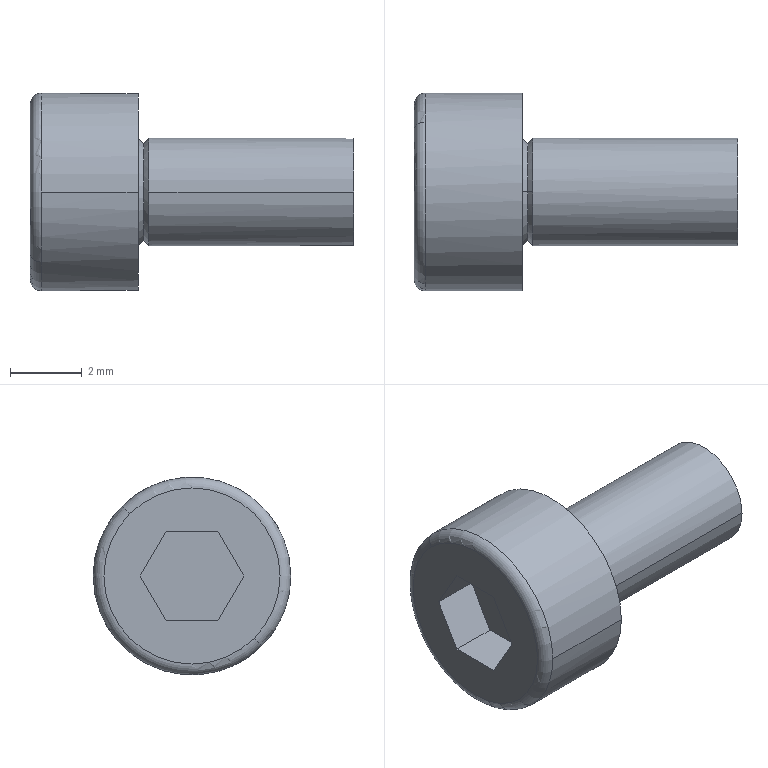Part | STEP file | ASND-0110-0211110400 | 1 solid | 20 faces | box 9 x 5.5 x 5.5 mm | volume 106.119 mm3 | plane 10 | cylinder 4 | cone 4 | torus 2 | commonest cylinder face diameters 3 x2 5.5 x2
STEP:
#1=CARTESIAN_POINT('',(0.,0.,0.));
#2=DIRECTION('',(0.,0.,1.));
#3=DIRECTION('',(1.,0.,0.));
#4=AXIS2_PLACEMENT_3D('',#1,#2,#3);
#5=CARTESIAN_POINT('',(-3.,-1.732,-1.732));
#6=VERTEX_POINT('',#5);
#7=CARTESIAN_POINT('',(-3.,1.732,1.732));
#8=VERTEX_POINT('',#7);
#9=CARTESIAN_POINT('',(-3.,0.,0.));
#10=DIRECTION('',(-1.,0.,0.));
#11=DIRECTION('',(0.,-1.,0.));
#12=AXIS2_PLACEMENT_3D('',#9,#10,#11);
#13=CIRCLE('',#12,2.45);
#14=CARTESIAN_POINT('',(-2.7,0.,0.));
#15=DIRECTION('',(1.,0.,0.));
#16=DIRECTION('',(0.,0.7071,0.7071));
#17=AXIS2_PLACEMENT_3D('',#14,#15,#16);
#18=TOROIDAL_SURFACE('',#17,2.45,0.3);
#19=CARTESIAN_POINT('',(8.639,4.712));
#20=DIRECTION('',(-1.,0.));
#21=VECTOR('',#20,1.);
#22=LINE('',#19,#21);
#23=(GEOMETRIC_REPRESENTATION_CONTEXT(2)PARAMETRIC_REPRESENTATION_CONTEXT()REPRESENTATION_CONTEXT('',''));
#24=DEFINITIONAL_REPRESENTATION('',(#22),#23);
#25=PCURVE('',#18,#24);
#26=CARTESIAN_POINT('',(-3.,0.,0.));
#27=DIRECTION('',(1.,0.,0.));
#28=DIRECTION('',(0.,0.7071,0.7071));
#29=AXIS2_PLACEMENT_3D('',#26,#27,#28);
#30=PLANE('',#29);
#31=CARTESIAN_POINT('',(-1.732,1.732));
#32=CARTESIAN_POINT('',(1.268,4.733));
#33=CARTESIAN_POINT('',(2.367,0.6341));
#34=CARTESIAN_POINT('',(3.465,-3.465));
#35=CARTESIAN_POINT('',(-0.6341,-2.367));
#36=CARTESIAN_POINT('',(-4.733,-1.268));
#37=CARTESIAN_POINT('',(-1.732,1.732));
#38=(BOUNDED_CURVE()B_SPLINE_CURVE(2,(#31,#32,#33,#34,#35,#36,#37),.UNSPECIFIED.,.T.,.F.)B_SPLINE_CURVE_WITH_KNOTS((1,2,2,2,2,1),(-2.094,0.,2.094,4.189,6.283,8.378),.UNSPECIFIED.)CURVE()GEOMETRIC_REPRESENTATION_ITEM()RATIONAL_B_SPLINE_CURVE((1.,0.5,1.,0.5,1.,0.5,1.))REPRESENTATION_ITEM(''));
#39=(GEOMETRIC_REPRESENTATION_CONTEXT(2)PARAMETRIC_REPRESENTATION_CONTEXT()REPRESENTATION_CONTEXT('',''));
#40=DEFINITIONAL_REPRESENTATION('',(#38),#39);
#41=PCURVE('',#30,#40);
#42=SURFACE_CURVE('',#13,(#25,#41),.PCURVE_S1.);
#43=EDGE_CURVE('',#6,#8,#42,.T.);
#44=ORIENTED_EDGE('',*,*,#43,.F.);
#45=CARTESIAN_POINT('',(-2.7,-1.945,-1.945));
#46=VERTEX_POINT('',#45);
#47=CARTESIAN_POINT('',(-2.7,-1.732,-1.732));
#48=DIRECTION('',(0.,-0.7071,0.7071));
#49=DIRECTION('',(0.,-0.7071,-0.7071));
#50=AXIS2_PLACEMENT_3D('',#47,#48,#49);
#51=CIRCLE('',#50,0.3);
#52=CARTESIAN_POINT('',(3.142,0.));
#53=DIRECTION('',(0.,1.));
#54=VECTOR('',#53,1.);
#55=LINE('',#52,#54);
#56=(GEOMETRIC_REPRESENTATION_CONTEXT(2)PARAMETRIC_REPRESENTATION_CONTEXT()REPRESENTATION_CONTEXT('',''));
#57=DEFINITIONAL_REPRESENTATION('',(#55),#56);
#58=PCURVE('',#18,#57);
#59=CARTESIAN_POINT('',(-2.7,0.,0.));
#60=DIRECTION('',(1.,0.,0.));
#61=DIRECTION('',(0.,0.7071,0.7071));
#62=AXIS2_PLACEMENT_3D('',#59,#60,#61);
#63=TOROIDAL_SURFACE('',#62,2.45,0.3);
#64=CARTESIAN_POINT('',(3.142,0.));
#65=DIRECTION('',(0.,1.));
#66=VECTOR('',#65,1.);
#67=LINE('',#64,#66);
#68=(GEOMETRIC_REPRESENTATION_CONTEXT(2)PARAMETRIC_REPRESENTATION_CONTEXT()REPRESENTATION_CONTEXT('',''));
#69=DEFINITIONAL_REPRESENTATION('',(#67),#68);
#70=PCURVE('',#63,#69);
#71=SURFACE_CURVE('',#51,(#58,#70),.PCURVE_S1.);
#72=EDGE_CURVE('',#6,#46,#71,.T.);
#73=ORIENTED_EDGE('',*,*,#72,.T.);
#74=CARTESIAN_POINT('',(-2.7,-2.75,0.));
#75=VERTEX_POINT('',#74);
#76=CARTESIAN_POINT('',(-2.7,0.,0.));
#77=DIRECTION('',(-1.,0.,0.));
#78=DIRECTION('',(0.,-1.,0.));
#79=AXIS2_PLACEMENT_3D('',#76,#77,#78);
#80=CIRCLE('',#79,2.75);
#81=CARTESIAN_POINT('',(8.639,6.283));
#82=DIRECTION('',(-1.,0.));
#83=VECTOR('',#82,1.);
#84=LINE('',#81,#83);
#85=(GEOMETRIC_REPRESENTATION_CONTEXT(2)PARAMETRIC_REPRESENTATION_CONTEXT()REPRESENTATION_CONTEXT('',''));
#86=DEFINITIONAL_REPRESENTATION('',(#84),#85);
#87=PCURVE('',#18,#86);
#88=CARTESIAN_POINT('',(-3.45,0.,0.));
#89=DIRECTION('',(1.,0.,0.));
#90=DIRECTION('',(0.,1.,0.));
#91=AXIS2_PLACEMENT_3D('',#88,#89,#90);
#92=CYLINDRICAL_SURFACE('',#91,2.75);
#93=CARTESIAN_POINT('',(9.425,0.75));
#94=DIRECTION('',(-1.,0.));
#95=VECTOR('',#94,1.);
#96=LINE('',#93,#95);
#97=(GEOMETRIC_REPRESENTATION_CONTEXT(2)PARAMETRIC_REPRESENTATION_CONTEXT()REPRESENTATION_CONTEXT('',''));
#98=DEFINITIONAL_REPRESENTATION('',(#96),#97);
#99=PCURVE('',#92,#98);
#100=SURFACE_CURVE('',#80,(#87,#99),.PCURVE_S1.);
#101=EDGE_CURVE('',#46,#75,#100,.T.);
#102=ORIENTED_EDGE('',*,*,#101,.T.);
#103=CARTESIAN_POINT('',(-2.7,1.945,1.945));
#104=VERTEX_POINT('',#103);
#105=CARTESIAN_POINT('',(-2.7,0.,0.));
#106=DIRECTION('',(-1.,0.,0.));
#107=DIRECTION('',(0.,-1.,0.));
#108=AXIS2_PLACEMENT_3D('',#105,#106,#107);
#109=CIRCLE('',#108,2.75);
#110=CARTESIAN_POINT('',(2.356,6.283));
#111=DIRECTION('',(-1.,0.));
#112=VECTOR('',#111,1.);
#113=LINE('',#110,#112);
#114=(GEOMETRIC_REPRESENTATION_CONTEXT(2)PARAMETRIC_REPRESENTATION_CONTEXT()REPRESENTATION_CONTEXT('',''));
#115=DEFINITIONAL_REPRESENTATION('',(#113),#114);
#116=PCURVE('',#18,#115);
#117=CARTESIAN_POINT('',(-3.45,0.,0.));
#118=DIRECTION('',(1.,0.,0.));
#119=DIRECTION('',(0.,1.,0.));
#120=AXIS2_PLACEMENT_3D('',#117,#118,#119);
#121=CYLINDRICAL_SURFACE('',#120,2.75);
#122=CARTESIAN_POINT('',(3.142,0.75));
#123=DIRECTION('',(-1.,0.));
#124=VECTOR('',#123,1.);
#125=LINE('',#122,#124);
#126=(GEOMETRIC_REPRESENTATION_CONTEXT(2)PARAMETRIC_REPRESENTATION_CONTEXT()REPRESENTATION_CONTEXT('',''));
#127=DEFINITIONAL_REPRESENTATION('',(#125),#126);
#128=PCURVE('',#121,#127);
#129=SURFACE_CURVE('',#109,(#116,#128),.PCURVE_S1.);
#130=EDGE_CURVE('',#75,#104,#129,.T.);
#131=ORIENTED_EDGE('',*,*,#130,.T.);
#132=CARTESIAN_POINT('',(-2.7,1.732,1.732));
#133=DIRECTION('',(0.,0.7071,-0.7071));
#134=DIRECTION('',(0.,0.7071,0.7071));
#135=AXIS2_PLACEMENT_3D('',#132,#133,#134);
#136=CIRCLE('',#135,0.3);
#137=CARTESIAN_POINT('',(0.,0.));
#138=DIRECTION('',(0.,1.));
#139=VECTOR('',#138,1.);
#140=LINE('',#137,#139);
#141=(GEOMETRIC_REPRESENTATION_CONTEXT(2)PARAMETRIC_REPRESENTATION_CONTEXT()REPRESENTATION_CONTEXT('',''));
#142=DEFINITIONAL_REPRESENTATION('',(#140),#141);
#143=PCURVE('',#18,#142);
#144=CARTESIAN_POINT('',(6.283,0.));
#145=DIRECTION('',(0.,1.));
#146=VECTOR('',#145,1.);
#147=LINE('',#144,#146);
#148=(GEOMETRIC_REPRESENTATION_CONTEXT(2)PARAMETRIC_REPRESENTATION_CONTEXT()REPRESENTATION_CONTEXT('',''));
#149=DEFINITIONAL_REPRESENTATION('',(#147),#148);
#150=PCURVE('',#63,#149);
#151=SURFACE_CURVE('',#136,(#143,#150),.PCURVE_S1.);
#152=EDGE_CURVE('',#8,#104,#151,.T.);
#153=ORIENTED_EDGE('',*,*,#152,.F.);
#154=EDGE_LOOP('',(#44,#73,#102,#131,#153));
#155=FACE_BOUND('',#154,.T.);
#156=ADVANCED_FACE('',(#155),#18,.T.);
#157=ORIENTED_EDGE('',*,*,#130,.F.);
#158=CARTESIAN_POINT('',(0.,-2.75,0.));
#159=VERTEX_POINT('',#158);
#160=CARTESIAN_POINT('',(-3.45,-2.75,0.));
#161=DIRECTION('',(1.,0.,0.));
#162=VECTOR('',#161,1.);
#163=LINE('',#160,#162);
#164=CARTESIAN_POINT('',(3.142,0.));
#165=DIRECTION('',(0.,1.));
#166=VECTOR('',#165,1.);
#167=LINE('',#164,#166);
#168=(GEOMETRIC_REPRESENTATION_CONTEXT(2)PARAMETRIC_REPRESENTATION_CONTEXT()REPRESENTATION_CONTEXT('',''));
#169=DEFINITIONAL_REPRESENTATION('',(#167),#168);
#170=PCURVE('',#121,#169);
#171=CARTESIAN_POINT('',(3.142,0.));
#172=DIRECTION('',(0.,1.));
#173=VECTOR('',#172,1.);
#174=LINE('',#171,#173);
#175=(GEOMETRIC_REPRESENTATION_CONTEXT(2)PARAMETRIC_REPRESENTATION_CONTEXT()REPRESENTATION_CONTEXT('',''));
#176=DEFINITIONAL_REPRESENTATION('',(#174),#175);
#177=PCURVE('',#92,#176);
#178=SURFACE_CURVE('',#163,(#170,#177),.PCURVE_S1.);
#179=EDGE_CURVE('',#75,#159,#178,.T.);
#180=ORIENTED_EDGE('',*,*,#179,.T.);
#181=CARTESIAN_POINT('',(0.,2.75,0.));
#182=VERTEX_POINT('',#181);
#183=CARTESIAN_POINT('',(0.,0.,0.));
#184=DIRECTION('',(-1.,0.,0.));
#185=DIRECTION('',(0.,-1.,0.));
#186=AXIS2_PLACEMENT_3D('',#183,#184,#185);
#187=CIRCLE('',#186,2.75);
#188=CARTESIAN_POINT('',(3.142,3.45));
#189=DIRECTION('',(-1.,0.));
#190=VECTOR('',#189,1.);
#191=LINE('',#188,#190);
#192=(GEOMETRIC_REPRESENTATION_CONTEXT(2)PARAMETRIC_REPRESENTATION_CONTEXT()REPRESENTATION_CONTEXT('',''));
#193=DEFINITIONAL_REPRESENTATION('',(#191),#192);
#194=PCURVE('',#121,#193);
#195=CARTESIAN_POINT('',(0.,0.,0.));
#196=DIRECTION('',(1.,0.,0.));
#197=DIRECTION('',(0.,0.7071,0.7071));
#198=AXIS2_PLACEMENT_3D('',#195,#196,#197);
#199=PLANE('',#198);
#200=CARTESIAN_POINT('',(-1.945,1.945));
#201=CARTESIAN_POINT('',(1.424,5.313));
#202=CARTESIAN_POINT('',(2.656,0.7118));
#203=CARTESIAN_POINT('',(3.889,-3.889));
#204=CARTESIAN_POINT('',(-0.7118,-2.656));
#205=CARTESIAN_POINT('',(-5.313,-1.424));
#206=CARTESIAN_POINT('',(-1.945,1.945));
#207=(BOUNDED_CURVE()B_SPLINE_CURVE(2,(#200,#201,#202,#203,#204,#205,#206),.UNSPECIFIED.,.T.,.F.)B_SPLINE_CURVE_WITH_KNOTS((1,2,2,2,2,1),(-2.094,0.,2.094,4.189,6.283,8.378),.UNSPECIFIED.)CURVE()GEOMETRIC_REPRESENTATION_ITEM()RATIONAL_B_SPLINE_CURVE((1.,0.5,1.,0.5,1.,0.5,1.))REPRESENTATION_ITEM(''));
#208=(GEOMETRIC_REPRESENTATION_CONTEXT(2)PARAMETRIC_REPRESENTATION_CONTEXT()REPRESENTATION_CONTEXT('',''));
#209=DEFINITIONAL_REPRESENTATION('',(#207),#208);
#210=PCURVE('',#199,#209);
#211=SURFACE_CURVE('',#187,(#194,#210),.PCURVE_S1.);
#212=EDGE_CURVE('',#159,#182,#211,.T.);
#213=ORIENTED_EDGE('',*,*,#212,.T.);
#214=CARTESIAN_POINT('',(-2.7,2.75,0.));
#215=VERTEX_POINT('',#214);
#216=CARTESIAN_POINT('',(-3.45,2.75,0.));
#217=DIRECTION('',(1.,0.,0.));
#218=VECTOR('',#217,1.);
#219=LINE('',#216,#218);
#220=CARTESIAN_POINT('',(0.,0.));
#221=DIRECTION('',(0.,1.));
#222=VECTOR('',#221,1.);
#223=LINE('',#220,#222);
#224=(GEOMETRIC_REPRESENTATION_CONTEXT(2)PARAMETRIC_REPRESENTATION_CONTEXT()REPRESENTATION_CONTEXT('',''));
#225=DEFINITIONAL_REPRESENTATION('',(#223),#224);
#226=PCURVE('',#121,#225);
#227=CARTESIAN_POINT('',(6.283,0.));
#228=DIRECTION('',(0.,1.));
#229=VECTOR('',#228,1.);
#230=LINE('',#227,#229);
#231=(GEOMETRIC_REPRESENTATION_CONTEXT(2)PARAMETRIC_REPRESENTATION_CONTEXT()REPRESENTATION_CONTEXT('',''));
#232=DEFINITIONAL_REPRESENTATION('',(#230),#231);
#233=PCURVE('',#92,#232);
#234=SURFACE_CURVE('',#219,(#226,#233),.PCURVE_S1.);
#235=EDGE_CURVE('',#215,#182,#234,.T.);
#236=ORIENTED_EDGE('',*,*,#235,.F.);
#237=CARTESIAN_POINT('',(-2.7,0.,0.));
#238=DIRECTION('',(-1.,0.,0.));
#239=DIRECTION('',(0.,-1.,0.));
#240=AXIS2_PLACEMENT_3D('',#237,#238,#239);
#241=CIRCLE('',#240,2.75);
#242=CARTESIAN_POINT('',(3.142,0.75));
#243=DIRECTION('',(-1.,0.));
#244=VECTOR('',#243,1.);
#245=LINE('',#242,#244);
#246=(GEOMETRIC_REPRESENTATION_CONTEXT(2)PARAMETRIC_REPRESENTATION_CONTEXT()REPRESENTATION_CONTEXT('',''));
#247=DEFINITIONAL_REPRESENTATION('',(#245),#246);
#248=PCURVE('',#121,#247);
#249=CARTESIAN_POINT('',(8.639,6.283));
#250=DIRECTION('',(-1.,0.));
#251=VECTOR('',#250,1.);
#252=LINE('',#249,#251);
#253=(GEOMETRIC_REPRESENTATION_CONTEXT(2)PARAMETRIC_REPRESENTATION_CONTEXT()REPRESENTATION_CONTEXT('',''));
#254=DEFINITIONAL_REPRESENTATION('',(#252),#253);
#255=PCURVE('',#63,#254);
#256=SURFACE_CURVE('',#241,(#248,#255),.PCURVE_S1.);
#257=EDGE_CURVE('',#104,#215,#256,.T.);
#258=ORIENTED_EDGE('',*,*,#257,.F.);
#259=EDGE_LOOP('',(#157,#180,#213,#236,#258));
#260=FACE_BOUND('',#259,.T.);
#261=ADVANCED_FACE('',(#260),#121,.T.);
#262=CARTESIAN_POINT('',(0.15,0.,-1.35));
#263=VERTEX_POINT('',#262);
#264=CARTESIAN_POINT('',(0.15,0.,1.35));
#265=VERTEX_POINT('',#264);
#266=CARTESIAN_POINT('',(0.15,0.,0.));
#267=DIRECTION('',(-1.,0.,0.));
#268=DIRECTION('',(0.,0.,-1.));
#269=AXIS2_PLACEMENT_3D('',#266,#267,#268);
#270=CIRCLE('',#269,1.35);
#271=CARTESIAN_POINT('',(0.075,0.,0.));
#272=DIRECTION('',(-1.,0.,0.));
#273=DIRECTION('',(0.,0.,-1.));
#274=AXIS2_PLACEMENT_3D('',#271,#272,#273);
#275=CONICAL_SURFACE('',#274,1.425,0.7854);
#276=CARTESIAN_POINT('',(0.,-0.075));
#277=DIRECTION('',(1.,0.));
#278=VECTOR('',#277,1.);
#279=LINE('',#276,#278);
#280=(GEOMETRIC_REPRESENTATION_CONTEXT(2)PARAMETRIC_REPRESENTATION_CONTEXT()REPRESENTATION_CONTEXT('',''));
#281=DEFINITIONAL_REPRESENTATION('',(#279),#280);
#282=PCURVE('',#275,#281);
#283=CARTESIAN_POINT('',(0.225,0.,0.));
#284=DIRECTION('',(1.,0.,0.));
#285=DIRECTION('',(0.,0.,1.));
#286=AXIS2_PLACEMENT_3D('',#283,#284,#285);
#287=CONICAL_SURFACE('',#286,1.425,0.7854);
#288=CARTESIAN_POINT('',(3.142,-0.075));
#289=DIRECTION('',(-1.,0.));
#290=VECTOR('',#289,1.);
#291=LINE('',#288,#290);
#292=(GEOMETRIC_REPRESENTATION_CONTEXT(2)PARAMETRIC_REPRESENTATION_CONTEXT()REPRESENTATION_CONTEXT('',''));
#293=DEFINITIONAL_REPRESENTATION('',(#291),#292);
#294=PCURVE('',#287,#293);
#295=SURFACE_CURVE('',#270,(#282,#294),.PCURVE_S1.);
#296=EDGE_CURVE('',#263,#265,#295,.T.);
#297=ORIENTED_EDGE('',*,*,#296,.T.);
#298=CARTESIAN_POINT('',(0.,0.,1.5));
#299=VERTEX_POINT('',#298);
#300=CARTESIAN_POINT('',(0.075,0.,1.425));
#301=DIRECTION('',(-0.7071,0.,0.7071));
#302=VECTOR('',#301,1.);
#303=LINE('',#300,#302);
#304=CARTESIAN_POINT('',(3.142,0.));
#305=DIRECTION('',(0.,1.));
#306=VECTOR('',#305,1.);
#307=LINE('',#304,#306);
#308=(GEOMETRIC_REPRESENTATION_CONTEXT(2)PARAMETRIC_REPRESENTATION_CONTEXT()REPRESENTATION_CONTEXT('',''));
#309=DEFINITIONAL_REPRESENTATION('',(#307),#308);
#310=PCURVE('',#275,#309);
#311=CARTESIAN_POINT('',(0.075,0.,0.));
#312=DIRECTION('',(-1.,0.,0.));
#313=DIRECTION('',(0.,0.,-1.));
#314=AXIS2_PLACEMENT_3D('',#311,#312,#313);
#315=CONICAL_SURFACE('',#314,1.425,0.7854);
#316=CARTESIAN_POINT('',(3.142,0.));
#317=DIRECTION('',(0.,1.));
#318=VECTOR('',#317,1.);
#319=LINE('',#316,#318);
#320=(GEOMETRIC_REPRESENTATION_CONTEXT(2)PARAMETRIC_REPRESENTATION_CONTEXT()REPRESENTATION_CONTEXT('',''));
#321=DEFINITIONAL_REPRESENTATION('',(#319),#320);
#322=PCURVE('',#315,#321);
#323=SURFACE_CURVE('',#303,(#310,#322),.PCURVE_S1.);
#324=EDGE_CURVE('',#265,#299,#323,.T.);
#325=ORIENTED_EDGE('',*,*,#324,.T.);
#326=CARTESIAN_POINT('',(0.,0.,-1.5));
#327=VERTEX_POINT('',#326);
#328=CARTESIAN_POINT('',(0.,0.,0.));
#329=DIRECTION('',(1.,0.,0.));
#330=DIRECTION('',(0.,0.,-1.));
#331=AXIS2_PLACEMENT_3D('',#328,#329,#330);
#332=CIRCLE('',#331,1.5);
#333=CARTESIAN_POINT('',(6.283,0.075));
#334=DIRECTION('',(-1.,0.));
#335=VECTOR('',#334,1.);
#336=LINE('',#333,#335);
#337=(GEOMETRIC_REPRESENTATION_CONTEXT(2)PARAMETRIC_REPRESENTATION_CONTEXT()REPRESENTATION_CONTEXT('',''));
#338=DEFINITIONAL_REPRESENTATION('',(#336),#337);
#339=PCURVE('',#275,#338);
#340=CARTESIAN_POINT('',(0.,0.));
#341=DIRECTION('',(-0.7071,-0.7071));
#342=AXIS2_PLACEMENT_2D('',#340,#341);
#343=CIRCLE('',#342,1.5);
#344=(GEOMETRIC_REPRESENTATION_CONTEXT(2)PARAMETRIC_REPRESENTATION_CONTEXT()REPRESENTATION_CONTEXT('',''));
#345=DEFINITIONAL_REPRESENTATION('',(#343),#344);
#346=PCURVE('',#199,#345);
#347=SURFACE_CURVE('',#332,(#339,#346),.PCURVE_S1.);
#348=EDGE_CURVE('',#299,#327,#347,.T.);
#349=ORIENTED_EDGE('',*,*,#348,.T.);
#350=CARTESIAN_POINT('',(0.075,0.,-1.425));
#351=DIRECTION('',(-0.7071,0.,-0.7071));
#352=VECTOR('',#351,1.);
#353=LINE('',#350,#352);
#354=CARTESIAN_POINT('',(0.,0.));
#355=DIRECTION('',(0.,1.));
#356=VECTOR('',#355,1.);
#357=LINE('',#354,#356);
#358=(GEOMETRIC_REPRESENTATION_CONTEXT(2)PARAMETRIC_REPRESENTATION_CONTEXT()REPRESENTATION_CONTEXT('',''));
#359=DEFINITIONAL_REPRESENTATION('',(#357),#358);
#360=PCURVE('',#275,#359);
#361=CARTESIAN_POINT('',(6.283,0.));
#362=DIRECTION('',(0.,1.));
#363=VECTOR('',#362,1.);
#364=LINE('',#361,#363);
#365=(GEOMETRIC_REPRESENTATION_CONTEXT(2)PARAMETRIC_REPRESENTATION_CONTEXT()REPRESENTATION_CONTEXT('',''));
#366=DEFINITIONAL_REPRESENTATION('',(#364),#365);
#367=PCURVE('',#315,#366);
#368=SURFACE_CURVE('',#353,(#360,#367),.PCURVE_S1.);
#369=EDGE_CURVE('',#263,#327,#368,.T.);
#370=ORIENTED_EDGE('',*,*,#369,.F.);
#371=EDGE_LOOP('',(#297,#325,#349,#370));
#372=FACE_BOUND('',#371,.T.);
#373=ADVANCED_FACE('',(#372),#275,.T.);
#374=ORIENTED_EDGE('',*,*,#296,.F.);
#375=CARTESIAN_POINT('',(0.3,0.,-1.5));
#376=VERTEX_POINT('',#375);
#377=CARTESIAN_POINT('',(0.225,0.,-1.425));
#378=DIRECTION('',(0.7071,0.,-0.7071));
#379=VECTOR('',#378,1.);
#380=LINE('',#377,#379);
#381=CARTESIAN_POINT('',(3.142,0.));
#382=DIRECTION('',(0.,1.));
#383=VECTOR('',#382,1.);
#384=LINE('',#381,#383);
#385=(GEOMETRIC_REPRESENTATION_CONTEXT(2)PARAMETRIC_REPRESENTATION_CONTEXT()REPRESENTATION_CONTEXT('',''));
#386=DEFINITIONAL_REPRESENTATION('',(#384),#385);
#387=PCURVE('',#287,#386);
#388=CARTESIAN_POINT('',(0.225,0.,0.));
#389=DIRECTION('',(1.,0.,0.));
#390=DIRECTION('',(0.,0.,1.));
#391=AXIS2_PLACEMENT_3D('',#388,#389,#390);
#392=CONICAL_SURFACE('',#391,1.425,0.7854);
#393=CARTESIAN_POINT('',(3.142,0.));
#394=DIRECTION('',(0.,1.));
#395=VECTOR('',#394,1.);
#396=LINE('',#393,#395);
#397=(GEOMETRIC_REPRESENTATION_CONTEXT(2)PARAMETRIC_REPRESENTATION_CONTEXT()REPRESENTATION_CONTEXT('',''));
#398=DEFINITIONAL_REPRESENTATION('',(#396),#397);
#399=PCURVE('',#392,#398);
#400=SURFACE_CURVE('',#380,(#387,#399),.PCURVE_S1.);
#401=EDGE_CURVE('',#263,#376,#400,.T.);
#402=ORIENTED_EDGE('',*,*,#401,.T.);
#403=CARTESIAN_POINT('',(0.3,-1.5,0.));
#404=VERTEX_POINT('',#403);
#405=CARTESIAN_POINT('',(0.3,0.,0.));
#406=DIRECTION('',(1.,0.,0.));
#407=DIRECTION('',(0.,0.,1.));
#408=AXIS2_PLACEMENT_3D('',#405,#406,#407);
#409=CIRCLE('',#408,1.5);
#410=CARTESIAN_POINT('',(0.,0.075));
#411=DIRECTION('',(1.,0.));
#412=VECTOR('',#411,1.);
#413=LINE('',#410,#412);
#414=(GEOMETRIC_REPRESENTATION_CONTEXT(2)PARAMETRIC_REPRESENTATION_CONTEXT()REPRESENTATION_CONTEXT('',''));
#415=DEFINITIONAL_REPRESENTATION('',(#413),#414);
#416=PCURVE('',#287,#415);
#417=CARTESIAN_POINT('',(-3.45,0.,0.));
#418=DIRECTION('',(1.,0.,0.));
#419=DIRECTION('',(0.,1.,0.));
#420=AXIS2_PLACEMENT_3D('',#417,#418,#419);
#421=CYLINDRICAL_SURFACE('',#420,1.5);
#422=CARTESIAN_POINT('',(1.571,3.75));
#423=DIRECTION('',(1.,0.));
#424=VECTOR('',#423,1.);
#425=LINE('',#422,#424);
#426=(GEOMETRIC_REPRESENTATION_CONTEXT(2)PARAMETRIC_REPRESENTATION_CONTEXT()REPRESENTATION_CONTEXT('',''));
#427=DEFINITIONAL_REPRESENTATION('',(#425),#426);
#428=PCURVE('',#421,#427);
#429=SURFACE_CURVE('',#409,(#416,#428),.PCURVE_S1.);
#430=EDGE_CURVE('',#404,#376,#429,.T.);
#431=ORIENTED_EDGE('',*,*,#430,.F.);
#432=CARTESIAN_POINT('',(0.3,0.,1.5));
#433=VERTEX_POINT('',#432);
#434=CARTESIAN_POINT('',(0.3,0.,0.));
#435=DIRECTION('',(1.,0.,0.));
#436=DIRECTION('',(0.,0.,1.));
#437=AXIS2_PLACEMENT_3D('',#434,#435,#436);
#438=CIRCLE('',#437,1.5);
#439=CARTESIAN_POINT('',(0.,0.075));
#440=DIRECTION('',(1.,0.));
#441=VECTOR('',#440,1.);
#442=LINE('',#439,#441);
#443=(GEOMETRIC_REPRESENTATION_CONTEXT(2)PARAMETRIC_REPRESENTATION_CONTEXT()REPRESENTATION_CONTEXT('',''));
#444=DEFINITIONAL_REPRESENTATION('',(#442),#443);
#445=PCURVE('',#287,#444);
#446=CARTESIAN_POINT('',(-3.45,0.,0.));
#447=DIRECTION('',(1.,0.,0.));
#448=DIRECTION('',(0.,1.,0.));
#449=AXIS2_PLACEMENT_3D('',#446,#447,#448);
#450=CYLINDRICAL_SURFACE('',#449,1.5);
#451=CARTESIAN_POINT('',(1.571,3.75));
#452=DIRECTION('',(1.,0.));
#453=VECTOR('',#452,1.);
#454=LINE('',#451,#453);
#455=(GEOMETRIC_REPRESENTATION_CONTEXT(2)PARAMETRIC_REPRESENTATION_CONTEXT()REPRESENTATION_CONTEXT('',''));
#456=DEFINITIONAL_REPRESENTATION('',(#454),#455);
#457=PCURVE('',#450,#456);
#458=SURFACE_CURVE('',#438,(#445,#457),.PCURVE_S1.);
#459=EDGE_CURVE('',#433,#404,#458,.T.);
#460=ORIENTED_EDGE('',*,*,#459,.F.);
#461=CARTESIAN_POINT('',(0.225,0.,1.425));
#462=DIRECTION('',(0.7071,0.,0.7071));
#463=VECTOR('',#462,1.);
#464=LINE('',#461,#463);
#465=CARTESIAN_POINT('',(0.,0.));
#466=DIRECTION('',(0.,1.));
#467=VECTOR('',#466,1.);
#468=LINE('',#465,#467);
#469=(GEOMETRIC_REPRESENTATION_CONTEXT(2)PARAMETRIC_REPRESENTATION_CONTEXT()REPRESENTATION_CONTEXT('',''));
#470=DEFINITIONAL_REPRESENTATION('',(#468),#469);
#471=PCURVE('',#287,#470);
#472=CARTESIAN_POINT('',(6.283,0.));
#473=DIRECTION('',(0.,1.));
#474=VECTOR('',#473,1.);
#475=LINE('',#472,#474);
#476=(GEOMETRIC_REPRESENTATION_CONTEXT(2)PARAMETRIC_REPRESENTATION_CONTEXT()REPRESENTATION_CONTEXT('',''));
#477=DEFINITIONAL_REPRESENTATION('',(#475),#476);
#478=PCURVE('',#392,#477);
#479=SURFACE_CURVE('',#464,(#471,#478),.PCURVE_S1.);
#480=EDGE_CURVE('',#265,#433,#479,.T.);
#481=ORIENTED_EDGE('',*,*,#480,.F.);
#482=EDGE_LOOP('',(#374,#402,#431,#460,#481));
#483=FACE_BOUND('',#482,.T.);
#484=ADVANCED_FACE('',(#483),#287,.T.);
#485=CARTESIAN_POINT('',(0.3,1.5,0.));
#486=VERTEX_POINT('',#485);
#487=CARTESIAN_POINT('',(0.3,0.,0.));
#488=DIRECTION('',(1.,0.,0.));
#489=DIRECTION('',(0.,0.,1.));
#490=AXIS2_PLACEMENT_3D('',#487,#488,#489);
#491=CIRCLE('',#490,1.5);
#492=CARTESIAN_POINT('',(-4.712,3.75));
#493=DIRECTION('',(1.,0.));
#494=VECTOR('',#493,1.);
#495=LINE('',#492,#494);
#496=(GEOMETRIC_REPRESENTATION_CONTEXT(2)PARAMETRIC_REPRESENTATION_CONTEXT()REPRESENTATION_CONTEXT('',''));
#497=DEFINITIONAL_REPRESENTATION('',(#495),#496);
#498=PCURVE('',#450,#497);
#499=CARTESIAN_POINT('',(0.,0.075));
#500=DIRECTION('',(1.,0.));
#501=VECTOR('',#500,1.);
#502=LINE('',#499,#501);
#503=(GEOMETRIC_REPRESENTATION_CONTEXT(2)PARAMETRIC_REPRESENTATION_CONTEXT()REPRESENTATION_CONTEXT('',''));
#504=DEFINITIONAL_REPRESENTATION('',(#502),#503);
#505=PCURVE('',#392,#504);
#506=SURFACE_CURVE('',#491,(#498,#505),.PCURVE_S1.);
#507=EDGE_CURVE('',#486,#433,#506,.T.);
#508=ORIENTED_EDGE('',*,*,#507,.T.);
#509=ORIENTED_EDGE('',*,*,#459,.T.);
#510=CARTESIAN_POINT('',(6.,-1.5,0.));
#511=VERTEX_POINT('',#510);
#512=CARTESIAN_POINT('',(-3.45,-1.5,0.));
#513=DIRECTION('',(1.,0.,0.));
#514=VECTOR('',#513,1.);
#515=LINE('',#512,#514);
#516=CARTESIAN_POINT('',(3.142,0.));
#517=DIRECTION('',(0.,1.));
#518=VECTOR('',#517,1.);
#519=LINE('',#516,#518);
#520=(GEOMETRIC_REPRESENTATION_CONTEXT(2)PARAMETRIC_REPRESENTATION_CONTEXT()REPRESENTATION_CONTEXT('',''));
#521=DEFINITIONAL_REPRESENTATION('',(#519),#520);
#522=PCURVE('',#450,#521);
#523=CARTESIAN_POINT('',(3.142,0.));
#524=DIRECTION('',(0.,1.));
#525=VECTOR('',#524,1.);
#526=LINE('',#523,#525);
#527=(GEOMETRIC_REPRESENTATION_CONTEXT(2)PARAMETRIC_REPRESENTATION_CONTEXT()REPRESENTATION_CONTEXT('',''));
#528=DEFINITIONAL_REPRESENTATION('',(#526),#527);
#529=PCURVE('',#421,#528);
#530=SURFACE_CURVE('',#515,(#522,#529),.PCURVE_S1.);
#531=EDGE_CURVE('',#404,#511,#530,.T.);
#532=ORIENTED_EDGE('',*,*,#531,.T.);
#533=CARTESIAN_POINT('',(6.,1.5,0.));
#534=VERTEX_POINT('',#533);
#535=CARTESIAN_POINT('',(6.,0.,0.));
#536=DIRECTION('',(-1.,0.,0.));
#537=DIRECTION('',(0.,-1.,0.));
#538=AXIS2_PLACEMENT_3D('',#535,#536,#537);
#539=CIRCLE('',#538,1.5);
#540=CARTESIAN_POINT('',(3.142,9.45));
#541=DIRECTION('',(-1.,0.));
#542=VECTOR('',#541,1.);
#543=LINE('',#540,#542);
#544=(GEOMETRIC_REPRESENTATION_CONTEXT(2)PARAMETRIC_REPRESENTATION_CONTEXT()REPRESENTATION_CONTEXT('',''));
#545=DEFINITIONAL_REPRESENTATION('',(#543),#544);
#546=PCURVE('',#450,#545);
#547=CARTESIAN_POINT('',(6.,0.,0.));
#548=DIRECTION('',(1.,0.,0.));
#549=DIRECTION('',(0.,0.7071,0.7071));
#550=AXIS2_PLACEMENT_3D('',#547,#548,#549);
#551=PLANE('',#550);
#552=CARTESIAN_POINT('',(-1.061,1.061));
#553=CARTESIAN_POINT('',(0.7765,2.898));
#554=CARTESIAN_POINT('',(1.449,0.3882));
#555=CARTESIAN_POINT('',(2.121,-2.121));
#556=CARTESIAN_POINT('',(-0.3882,-1.449));
#557=CARTESIAN_POINT('',(-2.898,-0.7765));
#558=CARTESIAN_POINT('',(-1.061,1.061));
#559=(BOUNDED_CURVE()B_SPLINE_CURVE(2,(#552,#553,#554,#555,#556,#557,#558),.UNSPECIFIED.,.T.,.F.)B_SPLINE_CURVE_WITH_KNOTS((1,2,2,2,2,1),(-2.094,0.,2.094,4.189,6.283,8.378),.UNSPECIFIED.)CURVE()GEOMETRIC_REPRESENTATION_ITEM()RATIONAL_B_SPLINE_CURVE((1.,0.5,1.,0.5,1.,0.5,1.))REPRESENTATION_ITEM(''));
#560=(GEOMETRIC_REPRESENTATION_CONTEXT(2)PARAMETRIC_REPRESENTATION_CONTEXT()REPRESENTATION_CONTEXT('',''));
#561=DEFINITIONAL_REPRESENTATION('',(#559),#560);
#562=PCURVE('',#551,#561);
#563=SURFACE_CURVE('',#539,(#546,#562),.PCURVE_S1.);
#564=EDGE_CURVE('',#511,#534,#563,.T.);
#565=ORIENTED_EDGE('',*,*,#564,.T.);
#566=CARTESIAN_POINT('',(-3.45,1.5,0.));
#567=DIRECTION('',(1.,0.,0.));
#568=VECTOR('',#567,1.);
#569=LINE('',#566,#568);
#570=CARTESIAN_POINT('',(0.,0.));
#571=DIRECTION('',(0.,1.));
#572=VECTOR('',#571,1.);
#573=LINE('',#570,#572);
#574=(GEOMETRIC_REPRESENTATION_CONTEXT(2)PARAMETRIC_REPRESENTATION_CONTEXT()REPRESENTATION_CONTEXT('',''));
#575=DEFINITIONAL_REPRESENTATION('',(#573),#574);
#576=PCURVE('',#450,#575);
#577=CARTESIAN_POINT('',(6.283,0.));
#578=DIRECTION('',(0.,1.));
#579=VECTOR('',#578,1.);
#580=LINE('',#577,#579);
#581=(GEOMETRIC_REPRESENTATION_CONTEXT(2)PARAMETRIC_REPRESENTATION_CONTEXT()REPRESENTATION_CONTEXT('',''));
#582=DEFINITIONAL_REPRESENTATION('',(#580),#581);
#583=PCURVE('',#421,#582);
#584=SURFACE_CURVE('',#569,(#576,#583),.PCURVE_S1.);
#585=EDGE_CURVE('',#486,#534,#584,.T.);
#586=ORIENTED_EDGE('',*,*,#585,.F.);
#587=EDGE_LOOP('',(#508,#509,#532,#565,#586));
#588=FACE_BOUND('',#587,.T.);
#589=ADVANCED_FACE('',(#588),#450,.T.);
#590=CARTESIAN_POINT('',(6.,0.,0.));
#591=DIRECTION('',(-1.,0.,0.));
#592=DIRECTION('',(0.,-1.,0.));
#593=AXIS2_PLACEMENT_3D('',#590,#591,#592);
#594=CIRCLE('',#593,1.5);
#595=CARTESIAN_POINT('',(-1.061,1.061));
#596=CARTESIAN_POINT('',(0.7765,2.898));
#597=CARTESIAN_POINT('',(1.449,0.3882));
#598=CARTESIAN_POINT('',(2.121,-2.121));
#599=CARTESIAN_POINT('',(-0.3882,-1.449));
#600=CARTESIAN_POINT('',(-2.898,-0.7765));
#601=CARTESIAN_POINT('',(-1.061,1.061));
#602=(BOUNDED_CURVE()B_SPLINE_CURVE(2,(#595,#596,#597,#598,#599,#600,#601),.UNSPECIFIED.,.T.,.F.)B_SPLINE_CURVE_WITH_KNOTS((1,2,2,2,2,1),(-2.094,0.,2.094,4.189,6.283,8.378),.UNSPECIFIED.)CURVE()GEOMETRIC_REPRESENTATION_ITEM()RATIONAL_B_SPLINE_CURVE((1.,0.5,1.,0.5,1.,0.5,1.))REPRESENTATION_ITEM(''));
#603=(GEOMETRIC_REPRESENTATION_CONTEXT(2)PARAMETRIC_REPRESENTATION_CONTEXT()REPRESENTATION_CONTEXT('',''));
#604=DEFINITIONAL_REPRESENTATION('',(#602),#603);
#605=PCURVE('',#551,#604);
#606=CARTESIAN_POINT('',(9.425,9.45));
#607=DIRECTION('',(-1.,0.));
#608=VECTOR('',#607,1.);
#609=LINE('',#606,#608);
#610=(GEOMETRIC_REPRESENTATION_CONTEXT(2)PARAMETRIC_REPRESENTATION_CONTEXT()REPRESENTATION_CONTEXT('',''));
#611=DEFINITIONAL_REPRESENTATION('',(#609),#610);
#612=PCURVE('',#421,#611);
#613=SURFACE_CURVE('',#594,(#605,#612),.PCURVE_S1.);
#614=EDGE_CURVE('',#534,#511,#613,.T.);
#615=ORIENTED_EDGE('',*,*,#614,.F.);
#616=ORIENTED_EDGE('',*,*,#564,.F.);
#617=EDGE_LOOP('',(#615,#616));
#618=FACE_BOUND('',#617,.T.);
#619=ADVANCED_FACE('',(#618),#551,.T.);
#620=ORIENTED_EDGE('',*,*,#531,.F.);
#621=ORIENTED_EDGE('',*,*,#430,.T.);
#622=CARTESIAN_POINT('',(0.3,0.,0.));
#623=DIRECTION('',(1.,0.,0.));
#624=DIRECTION('',(0.,0.,1.));
#625=AXIS2_PLACEMENT_3D('',#622,#623,#624);
#626=CIRCLE('',#625,1.5);
#627=CARTESIAN_POINT('',(1.571,3.75));
#628=DIRECTION('',(1.,0.));
#629=VECTOR('',#628,1.);
#630=LINE('',#627,#629);
#631=(GEOMETRIC_REPRESENTATION_CONTEXT(2)PARAMETRIC_REPRESENTATION_CONTEXT()REPRESENTATION_CONTEXT('',''));
#632=DEFINITIONAL_REPRESENTATION('',(#630),#631);
#633=PCURVE('',#421,#632);
#634=CARTESIAN_POINT('',(0.,0.075));
#635=DIRECTION('',(1.,0.));
#636=VECTOR('',#635,1.);
#637=LINE('',#634,#636);
#638=(GEOMETRIC_REPRESENTATION_CONTEXT(2)PARAMETRIC_REPRESENTATION_CONTEXT()REPRESENTATION_CONTEXT('',''));
#639=DEFINITIONAL_REPRESENTATION('',(#637),#638);
#640=PCURVE('',#392,#639);
#641=SURFACE_CURVE('',#626,(#633,#640),.PCURVE_S1.);
#642=EDGE_CURVE('',#376,#486,#641,.T.);
#643=ORIENTED_EDGE('',*,*,#642,.T.);
#644=ORIENTED_EDGE('',*,*,#585,.T.);
#645=ORIENTED_EDGE('',*,*,#614,.T.);
#646=EDGE_LOOP('',(#620,#621,#643,#644,#645));
#647=FACE_BOUND('',#646,.T.);
#648=ADVANCED_FACE('',(#647),#421,.T.);
#649=ORIENTED_EDGE('',*,*,#401,.F.);
#650=CARTESIAN_POINT('',(0.15,0.,0.));
#651=DIRECTION('',(-1.,0.,0.));
#652=DIRECTION('',(0.,0.,-1.));
#653=AXIS2_PLACEMENT_3D('',#650,#651,#652);
#654=CIRCLE('',#653,1.35);
#655=CARTESIAN_POINT('',(9.425,-0.075));
#656=DIRECTION('',(-1.,0.));
#657=VECTOR('',#656,1.);
#658=LINE('',#655,#657);
#659=(GEOMETRIC_REPRESENTATION_CONTEXT(2)PARAMETRIC_REPRESENTATION_CONTEXT()REPRESENTATION_CONTEXT('',''));
#660=DEFINITIONAL_REPRESENTATION('',(#658),#659);
#661=PCURVE('',#392,#660);
#662=CARTESIAN_POINT('',(0.,-0.075));
#663=DIRECTION('',(1.,0.));
#664=VECTOR('',#663,1.);
#665=LINE('',#662,#664);
#666=(GEOMETRIC_REPRESENTATION_CONTEXT(2)PARAMETRIC_REPRESENTATION_CONTEXT()REPRESENTATION_CONTEXT('',''));
#667=DEFINITIONAL_REPRESENTATION('',(#665),#666);
#668=PCURVE('',#315,#667);
#669=SURFACE_CURVE('',#654,(#661,#668),.PCURVE_S1.);
#670=EDGE_CURVE('',#265,#263,#669,.T.);
#671=ORIENTED_EDGE('',*,*,#670,.F.);
#672=ORIENTED_EDGE('',*,*,#480,.T.);
#673=ORIENTED_EDGE('',*,*,#507,.F.);
#674=ORIENTED_EDGE('',*,*,#642,.F.);
#675=EDGE_LOOP('',(#649,#671,#672,#673,#674));
#676=FACE_BOUND('',#675,.T.);
#677=ADVANCED_FACE('',(#676),#392,.T.);
#678=ORIENTED_EDGE('',*,*,#324,.F.);
#679=ORIENTED_EDGE('',*,*,#670,.T.);
#680=ORIENTED_EDGE('',*,*,#369,.T.);
#681=CARTESIAN_POINT('',(0.,0.,0.));
#682=DIRECTION('',(1.,0.,0.));
#683=DIRECTION('',(0.,0.,-1.));
#684=AXIS2_PLACEMENT_3D('',#681,#682,#683);
#685=CIRCLE('',#684,1.5);
#686=CARTESIAN_POINT('',(6.283,0.075));
#687=DIRECTION('',(-1.,0.));
#688=VECTOR('',#687,1.);
#689=LINE('',#686,#688);
#690=(GEOMETRIC_REPRESENTATION_CONTEXT(2)PARAMETRIC_REPRESENTATION_CONTEXT()REPRESENTATION_CONTEXT('',''));
#691=DEFINITIONAL_REPRESENTATION('',(#689),#690);
#692=PCURVE('',#315,#691);
#693=CARTESIAN_POINT('',(0.,0.));
#694=DIRECTION('',(-0.7071,-0.7071));
#695=AXIS2_PLACEMENT_2D('',#693,#694);
#696=CIRCLE('',#695,1.5);
#697=(GEOMETRIC_REPRESENTATION_CONTEXT(2)PARAMETRIC_REPRESENTATION_CONTEXT()REPRESENTATION_CONTEXT('',''));
#698=DEFINITIONAL_REPRESENTATION('',(#696),#697);
#699=PCURVE('',#199,#698);
#700=SURFACE_CURVE('',#685,(#692,#699),.PCURVE_S1.);
#701=EDGE_CURVE('',#327,#299,#700,.T.);
#702=ORIENTED_EDGE('',*,*,#701,.T.);
#703=EDGE_LOOP('',(#678,#679,#680,#702));
#704=FACE_BOUND('',#703,.T.);
#705=ADVANCED_FACE('',(#704),#315,.T.);
#706=CARTESIAN_POINT('',(0.,0.,0.));
#707=DIRECTION('',(-1.,0.,0.));
#708=DIRECTION('',(0.,-1.,0.));
#709=AXIS2_PLACEMENT_3D('',#706,#707,#708);
#710=CIRCLE('',#709,2.75);
#711=CARTESIAN_POINT('',(-1.945,1.945));
#712=CARTESIAN_POINT('',(1.424,5.313));
#713=CARTESIAN_POINT('',(2.656,0.7118));
#714=CARTESIAN_POINT('',(3.889,-3.889));
#715=CARTESIAN_POINT('',(-0.7118,-2.656));
#716=CARTESIAN_POINT('',(-5.313,-1.424));
#717=CARTESIAN_POINT('',(-1.945,1.945));
#718=(BOUNDED_CURVE()B_SPLINE_CURVE(2,(#711,#712,#713,#714,#715,#716,#717),.UNSPECIFIED.,.T.,.F.)B_SPLINE_CURVE_WITH_KNOTS((1,2,2,2,2,1),(-2.094,0.,2.094,4.189,6.283,8.378),.UNSPECIFIED.)CURVE()GEOMETRIC_REPRESENTATION_ITEM()RATIONAL_B_SPLINE_CURVE((1.,0.5,1.,0.5,1.,0.5,1.))REPRESENTATION_ITEM(''));
#719=(GEOMETRIC_REPRESENTATION_CONTEXT(2)PARAMETRIC_REPRESENTATION_CONTEXT()REPRESENTATION_CONTEXT('',''));
#720=DEFINITIONAL_REPRESENTATION('',(#718),#719);
#721=PCURVE('',#199,#720);
#722=CARTESIAN_POINT('',(9.425,3.45));
#723=DIRECTION('',(-1.,0.));
#724=VECTOR('',#723,1.);
#725=LINE('',#722,#724);
#726=(GEOMETRIC_REPRESENTATION_CONTEXT(2)PARAMETRIC_REPRESENTATION_CONTEXT()REPRESENTATION_CONTEXT('',''));
#727=DEFINITIONAL_REPRESENTATION('',(#725),#726);
#728=PCURVE('',#92,#727);
#729=SURFACE_CURVE('',#710,(#721,#728),.PCURVE_S1.);
#730=EDGE_CURVE('',#182,#159,#729,.T.);
#731=ORIENTED_EDGE('',*,*,#730,.F.);
#732=ORIENTED_EDGE('',*,*,#212,.F.);
#733=EDGE_LOOP('',(#731,#732));
#734=FACE_BOUND('',#733,.T.);
#735=ORIENTED_EDGE('',*,*,#701,.F.);
#736=ORIENTED_EDGE('',*,*,#348,.F.);
#737=EDGE_LOOP('',(#735,#736));
#738=FACE_BOUND('',#737,.T.);
#739=ADVANCED_FACE('',(#734,#738),#199,.T.);
#740=ORIENTED_EDGE('',*,*,#179,.F.);
#741=ORIENTED_EDGE('',*,*,#101,.F.);
#742=CARTESIAN_POINT('',(-2.7,0.,0.));
#743=DIRECTION('',(-1.,0.,0.));
#744=DIRECTION('',(0.,-1.,0.));
#745=AXIS2_PLACEMENT_3D('',#742,#743,#744);
#746=CIRCLE('',#745,2.75);
#747=CARTESIAN_POINT('',(9.425,0.75));
#748=DIRECTION('',(-1.,0.));
#749=VECTOR('',#748,1.);
#750=LINE('',#747,#749);
#751=(GEOMETRIC_REPRESENTATION_CONTEXT(2)PARAMETRIC_REPRESENTATION_CONTEXT()REPRESENTATION_CONTEXT('',''));
#752=DEFINITIONAL_REPRESENTATION('',(#750),#751);
#753=PCURVE('',#92,#752);
#754=CARTESIAN_POINT('',(8.639,6.283));
#755=DIRECTION('',(-1.,0.));
#756=VECTOR('',#755,1.);
#757=LINE('',#754,#756);
#758=(GEOMETRIC_REPRESENTATION_CONTEXT(2)PARAMETRIC_REPRESENTATION_CONTEXT()REPRESENTATION_CONTEXT('',''));
#759=DEFINITIONAL_REPRESENTATION('',(#757),#758);
#760=PCURVE('',#63,#759);
#761=SURFACE_CURVE('',#746,(#753,#760),.PCURVE_S1.);
#762=EDGE_CURVE('',#215,#46,#761,.T.);
#763=ORIENTED_EDGE('',*,*,#762,.F.);
#764=ORIENTED_EDGE('',*,*,#235,.T.);
#765=ORIENTED_EDGE('',*,*,#730,.T.);
#766=EDGE_LOOP('',(#740,#741,#763,#764,#765));
#767=FACE_BOUND('',#766,.T.);
#768=ADVANCED_FACE('',(#767),#92,.T.);
#769=ORIENTED_EDGE('',*,*,#72,.F.);
#770=CARTESIAN_POINT('',(-3.,0.,0.));
#771=DIRECTION('',(-1.,0.,0.));
#772=DIRECTION('',(0.,-1.,0.));
#773=AXIS2_PLACEMENT_3D('',#770,#771,#772);
#774=CIRCLE('',#773,2.45);
#775=CARTESIAN_POINT('',(8.639,4.712));
#776=DIRECTION('',(-1.,0.));
#777=VECTOR('',#776,1.);
#778=LINE('',#775,#777);
#779=(GEOMETRIC_REPRESENTATION_CONTEXT(2)PARAMETRIC_REPRESENTATION_CONTEXT()REPRESENTATION_CONTEXT('',''));
#780=DEFINITIONAL_REPRESENTATION('',(#778),#779);
#781=PCURVE('',#63,#780);
#782=CARTESIAN_POINT('',(-1.732,1.732));
#783=CARTESIAN_POINT('',(1.268,4.733));
#784=CARTESIAN_POINT('',(2.367,0.6341));
#785=CARTESIAN_POINT('',(3.465,-3.465));
#786=CARTESIAN_POINT('',(-0.6341,-2.367));
#787=CARTESIAN_POINT('',(-4.733,-1.268));
#788=CARTESIAN_POINT('',(-1.732,1.732));
#789=(BOUNDED_CURVE()B_SPLINE_CURVE(2,(#782,#783,#784,#785,#786,#787,#788),.UNSPECIFIED.,.T.,.F.)B_SPLINE_CURVE_WITH_KNOTS((1,2,2,2,2,1),(-2.094,0.,2.094,4.189,6.283,8.378),.UNSPECIFIED.)CURVE()GEOMETRIC_REPRESENTATION_ITEM()RATIONAL_B_SPLINE_CURVE((1.,0.5,1.,0.5,1.,0.5,1.))REPRESENTATION_ITEM(''));
#790=(GEOMETRIC_REPRESENTATION_CONTEXT(2)PARAMETRIC_REPRESENTATION_CONTEXT()REPRESENTATION_CONTEXT('',''));
#791=DEFINITIONAL_REPRESENTATION('',(#789),#790);
#792=PCURVE('',#30,#791);
#793=SURFACE_CURVE('',#774,(#781,#792),.PCURVE_S1.);
#794=EDGE_CURVE('',#8,#6,#793,.T.);
#795=ORIENTED_EDGE('',*,*,#794,.F.);
#796=ORIENTED_EDGE('',*,*,#152,.T.);
#797=ORIENTED_EDGE('',*,*,#257,.T.);
#798=ORIENTED_EDGE('',*,*,#762,.T.);
#799=EDGE_LOOP('',(#769,#795,#796,#797,#798));
#800=FACE_BOUND('',#799,.T.);
#801=ADVANCED_FACE('',(#800),#63,.T.);
#802=ORIENTED_EDGE('',*,*,#794,.T.);
#803=ORIENTED_EDGE('',*,*,#43,.T.);
#804=EDGE_LOOP('',(#802,#803));
#805=FACE_BOUND('',#804,.T.);
#806=CARTESIAN_POINT('',(-3.,0.7217,1.25));
#807=VERTEX_POINT('',#806);
#808=CARTESIAN_POINT('',(-3.,1.443,0.));
#809=VERTEX_POINT('',#808);
#810=CARTESIAN_POINT('',(-3.,0.7217,1.25));
#811=DIRECTION('',(0.,0.5,-0.866));
#812=VECTOR('',#811,1.);
#813=LINE('',#810,#812);
#814=CARTESIAN_POINT('',(1.394,0.3736));
#815=DIRECTION('',(-0.2588,-0.9659));
#816=VECTOR('',#815,1.);
#817=LINE('',#814,#816);
#818=(GEOMETRIC_REPRESENTATION_CONTEXT(2)PARAMETRIC_REPRESENTATION_CONTEXT()REPRESENTATION_CONTEXT('',''));
#819=DEFINITIONAL_REPRESENTATION('',(#817),#818);
#820=PCURVE('',#30,#819);
#821=CARTESIAN_POINT('',(-3.,0.7217,1.25));
#822=DIRECTION('',(0.,0.866,0.5));
#823=DIRECTION('',(0.6547,-0.378,0.6547));
#824=AXIS2_PLACEMENT_3D('',#821,#822,#823);
#825=PLANE('',#824);
#826=CARTESIAN_POINT('',(0.,0.));
#827=DIRECTION('',(-0.7559,0.6547));
#828=VECTOR('',#827,1.);
#829=LINE('',#826,#828);
#830=(GEOMETRIC_REPRESENTATION_CONTEXT(2)PARAMETRIC_REPRESENTATION_CONTEXT()REPRESENTATION_CONTEXT('',''));
#831=DEFINITIONAL_REPRESENTATION('',(#829),#830);
#832=PCURVE('',#825,#831);
#833=SURFACE_CURVE('',#813,(#820,#832),.PCURVE_S1.);
#834=EDGE_CURVE('',#807,#809,#833,.T.);
#835=ORIENTED_EDGE('',*,*,#834,.F.);
#836=CARTESIAN_POINT('',(-3.,-0.7217,1.25));
#837=VERTEX_POINT('',#836);
#838=CARTESIAN_POINT('',(-3.,-0.7217,1.25));
#839=DIRECTION('',(0.,1.,0.));
#840=VECTOR('',#839,1.);
#841=LINE('',#838,#840);
#842=CARTESIAN_POINT('',(0.3736,1.394));
#843=DIRECTION('',(0.7071,-0.7071));
#844=VECTOR('',#843,1.);
#845=LINE('',#842,#844);
#846=(GEOMETRIC_REPRESENTATION_CONTEXT(2)PARAMETRIC_REPRESENTATION_CONTEXT()REPRESENTATION_CONTEXT('',''));
#847=DEFINITIONAL_REPRESENTATION('',(#845),#846);
#848=PCURVE('',#30,#847);
#849=CARTESIAN_POINT('',(-3.,-0.7217,1.25));
#850=DIRECTION('',(0.,0.,1.));
#851=DIRECTION('',(0.7071,0.7071,0.));
#852=AXIS2_PLACEMENT_3D('',#849,#850,#851);
#853=PLANE('',#852);
#854=CARTESIAN_POINT('',(0.,0.));
#855=DIRECTION('',(0.7071,0.7071));
#856=VECTOR('',#855,1.);
#857=LINE('',#854,#856);
#858=(GEOMETRIC_REPRESENTATION_CONTEXT(2)PARAMETRIC_REPRESENTATION_CONTEXT()REPRESENTATION_CONTEXT('',''));
#859=DEFINITIONAL_REPRESENTATION('',(#857),#858);
#860=PCURVE('',#853,#859);
#861=SURFACE_CURVE('',#841,(#848,#860),.PCURVE_S1.);
#862=EDGE_CURVE('',#837,#807,#861,.T.);
#863=ORIENTED_EDGE('',*,*,#862,.F.);
#864=CARTESIAN_POINT('',(-3.,-1.443,0.));
#865=VERTEX_POINT('',#864);
#866=CARTESIAN_POINT('',(-3.,-1.443,0.));
#867=DIRECTION('',(0.,0.5,0.866));
#868=VECTOR('',#867,1.);
#869=LINE('',#866,#868);
#870=CARTESIAN_POINT('',(-1.021,1.021));
#871=DIRECTION('',(0.9659,0.2588));
#872=VECTOR('',#871,1.);
#873=LINE('',#870,#872);
#874=(GEOMETRIC_REPRESENTATION_CONTEXT(2)PARAMETRIC_REPRESENTATION_CONTEXT()REPRESENTATION_CONTEXT('',''));
#875=DEFINITIONAL_REPRESENTATION('',(#873),#874);
#876=PCURVE('',#30,#875);
#877=CARTESIAN_POINT('',(-3.,-1.443,0.));
#878=DIRECTION('',(0.,-0.866,0.5));
#879=DIRECTION('',(0.6547,0.378,0.6547));
#880=AXIS2_PLACEMENT_3D('',#877,#878,#879);
#881=PLANE('',#880);
#882=CARTESIAN_POINT('',(0.,0.));
#883=DIRECTION('',(0.7559,0.6547));
#884=VECTOR('',#883,1.);
#885=LINE('',#882,#884);
#886=(GEOMETRIC_REPRESENTATION_CONTEXT(2)PARAMETRIC_REPRESENTATION_CONTEXT()REPRESENTATION_CONTEXT('',''));
#887=DEFINITIONAL_REPRESENTATION('',(#885),#886);
#888=PCURVE('',#881,#887);
#889=SURFACE_CURVE('',#869,(#876,#888),.PCURVE_S1.);
#890=EDGE_CURVE('',#865,#837,#889,.T.);
#891=ORIENTED_EDGE('',*,*,#890,.F.);
#892=CARTESIAN_POINT('',(-3.,-0.7217,-1.25));
#893=VERTEX_POINT('',#892);
#894=CARTESIAN_POINT('',(-3.,-0.7217,-1.25));
#895=DIRECTION('',(0.,-0.5,0.866));
#896=VECTOR('',#895,1.);
#897=LINE('',#894,#896);
#898=CARTESIAN_POINT('',(-1.394,-0.3736));
#899=DIRECTION('',(0.2588,0.9659));
#900=VECTOR('',#899,1.);
#901=LINE('',#898,#900);
#902=(GEOMETRIC_REPRESENTATION_CONTEXT(2)PARAMETRIC_REPRESENTATION_CONTEXT()REPRESENTATION_CONTEXT('',''));
#903=DEFINITIONAL_REPRESENTATION('',(#901),#902);
#904=PCURVE('',#30,#903);
#905=CARTESIAN_POINT('',(-3.,-0.7217,-1.25));
#906=DIRECTION('',(0.,-0.866,-0.5));
#907=DIRECTION('',(0.6547,-0.378,0.6547));
#908=AXIS2_PLACEMENT_3D('',#905,#906,#907);
#909=PLANE('',#908);
#910=CARTESIAN_POINT('',(0.,0.));
#911=DIRECTION('',(0.7559,0.6547));
#912=VECTOR('',#911,1.);
#913=LINE('',#910,#912);
#914=(GEOMETRIC_REPRESENTATION_CONTEXT(2)PARAMETRIC_REPRESENTATION_CONTEXT()REPRESENTATION_CONTEXT('',''));
#915=DEFINITIONAL_REPRESENTATION('',(#913),#914);
#916=PCURVE('',#909,#915);
#917=SURFACE_CURVE('',#897,(#904,#916),.PCURVE_S1.);
#918=EDGE_CURVE('',#893,#865,#917,.T.);
#919=ORIENTED_EDGE('',*,*,#918,.F.);
#920=CARTESIAN_POINT('',(-3.,0.7217,-1.25));
#921=VERTEX_POINT('',#920);
#922=CARTESIAN_POINT('',(-3.,0.7217,-1.25));
#923=DIRECTION('',(0.,-1.,0.));
#924=VECTOR('',#923,1.);
#925=LINE('',#922,#924);
#926=CARTESIAN_POINT('',(-0.3736,-1.394));
#927=DIRECTION('',(-0.7071,0.7071));
#928=VECTOR('',#927,1.);
#929=LINE('',#926,#928);
#930=(GEOMETRIC_REPRESENTATION_CONTEXT(2)PARAMETRIC_REPRESENTATION_CONTEXT()REPRESENTATION_CONTEXT('',''));
#931=DEFINITIONAL_REPRESENTATION('',(#929),#930);
#932=PCURVE('',#30,#931);
#933=CARTESIAN_POINT('',(-3.,0.7217,-1.25));
#934=DIRECTION('',(0.,0.,-1.));
#935=DIRECTION('',(0.7071,0.7071,0.));
#936=AXIS2_PLACEMENT_3D('',#933,#934,#935);
#937=PLANE('',#936);
#938=CARTESIAN_POINT('',(0.,0.));
#939=DIRECTION('',(-0.7071,0.7071));
#940=VECTOR('',#939,1.);
#941=LINE('',#938,#940);
#942=(GEOMETRIC_REPRESENTATION_CONTEXT(2)PARAMETRIC_REPRESENTATION_CONTEXT()REPRESENTATION_CONTEXT('',''));
#943=DEFINITIONAL_REPRESENTATION('',(#941),#942);
#944=PCURVE('',#937,#943);
#945=SURFACE_CURVE('',#925,(#932,#944),.PCURVE_S1.);
#946=EDGE_CURVE('',#921,#893,#945,.T.);
#947=ORIENTED_EDGE('',*,*,#946,.F.);
#948=CARTESIAN_POINT('',(-3.,1.443,0.));
#949=DIRECTION('',(0.,-0.5,-0.866));
#950=VECTOR('',#949,1.);
#951=LINE('',#948,#950);
#952=CARTESIAN_POINT('',(1.021,-1.021));
#953=DIRECTION('',(-0.9659,-0.2588));
#954=VECTOR('',#953,1.);
#955=LINE('',#952,#954);
#956=(GEOMETRIC_REPRESENTATION_CONTEXT(2)PARAMETRIC_REPRESENTATION_CONTEXT()REPRESENTATION_CONTEXT('',''));
#957=DEFINITIONAL_REPRESENTATION('',(#955),#956);
#958=PCURVE('',#30,#957);
#959=CARTESIAN_POINT('',(-3.,1.443,0.));
#960=DIRECTION('',(0.,0.866,-0.5));
#961=DIRECTION('',(0.6547,0.378,0.6547));
#962=AXIS2_PLACEMENT_3D('',#959,#960,#961);
#963=PLANE('',#962);
#964=CARTESIAN_POINT('',(0.,0.));
#965=DIRECTION('',(-0.7559,0.6547));
#966=VECTOR('',#965,1.);
#967=LINE('',#964,#966);
#968=(GEOMETRIC_REPRESENTATION_CONTEXT(2)PARAMETRIC_REPRESENTATION_CONTEXT()REPRESENTATION_CONTEXT('',''));
#969=DEFINITIONAL_REPRESENTATION('',(#967),#968);
#970=PCURVE('',#963,#969);
#971=SURFACE_CURVE('',#951,(#958,#970),.PCURVE_S1.);
#972=EDGE_CURVE('',#809,#921,#971,.T.);
#973=ORIENTED_EDGE('',*,*,#972,.F.);
#974=EDGE_LOOP('',(#835,#863,#891,#919,#947,#973));
#975=FACE_BOUND('',#974,.T.);
#976=ADVANCED_FACE('',(#805,#975),#30,.F.);
#977=ORIENTED_EDGE('',*,*,#834,.T.);
#978=CARTESIAN_POINT('',(-1.7,1.443,0.));
#979=VERTEX_POINT('',#978);
#980=CARTESIAN_POINT('',(-3.,1.443,0.));
#981=DIRECTION('',(1.,0.,0.));
#982=VECTOR('',#981,1.);
#983=LINE('',#980,#982);
#984=CARTESIAN_POINT('',(-1.091,0.9449));
#985=DIRECTION('',(0.6547,0.7559));
#986=VECTOR('',#985,1.);
#987=LINE('',#984,#986);
#988=(GEOMETRIC_REPRESENTATION_CONTEXT(2)PARAMETRIC_REPRESENTATION_CONTEXT()REPRESENTATION_CONTEXT('',''));
#989=DEFINITIONAL_REPRESENTATION('',(#987),#988);
#990=PCURVE('',#825,#989);
#991=CARTESIAN_POINT('',(0.,0.));
#992=DIRECTION('',(0.6547,0.7559));
#993=VECTOR('',#992,1.);
#994=LINE('',#991,#993);
#995=(GEOMETRIC_REPRESENTATION_CONTEXT(2)PARAMETRIC_REPRESENTATION_CONTEXT()REPRESENTATION_CONTEXT('',''));
#996=DEFINITIONAL_REPRESENTATION('',(#994),#995);
#997=PCURVE('',#963,#996);
#998=SURFACE_CURVE('',#983,(#990,#997),.PCURVE_S1.);
#999=EDGE_CURVE('',#809,#979,#998,.T.);
#1000=ORIENTED_EDGE('',*,*,#999,.T.);
#1001=CARTESIAN_POINT('',(-1.7,0.7217,1.25));
#1002=VERTEX_POINT('',#1001);
#1003=CARTESIAN_POINT('',(-1.7,0.7217,1.25));
#1004=DIRECTION('',(0.,0.5,-0.866));
#1005=VECTOR('',#1004,1.);
#1006=LINE('',#1003,#1005);
#1007=CARTESIAN_POINT('',(0.851,0.9827));
#1008=DIRECTION('',(-0.7559,0.6547));
#1009=VECTOR('',#1008,1.);
#1010=LINE('',#1007,#1009);
#1011=(GEOMETRIC_REPRESENTATION_CONTEXT(2)PARAMETRIC_REPRESENTATION_CONTEXT()REPRESENTATION_CONTEXT('',''));
#1012=DEFINITIONAL_REPRESENTATION('',(#1010),#1011);
#1013=PCURVE('',#825,#1012);
#1014=CARTESIAN_POINT('',(-1.7,0.,0.));
#1015=DIRECTION('',(-1.,0.,0.));
#1016=DIRECTION('',(0.,0.7071,0.7071));
#1017=AXIS2_PLACEMENT_3D('',#1014,#1015,#1016);
#1018=PLANE('',#1017);
#1019=CARTESIAN_POINT('',(1.394,-0.3736));
#1020=DIRECTION('',(-0.2588,0.9659));
#1021=VECTOR('',#1020,1.);
#1022=LINE('',#1019,#1021);
#1023=(GEOMETRIC_REPRESENTATION_CONTEXT(2)PARAMETRIC_REPRESENTATION_CONTEXT()REPRESENTATION_CONTEXT('',''));
#1024=DEFINITIONAL_REPRESENTATION('',(#1022),#1023);
#1025=PCURVE('',#1018,#1024);
#1026=SURFACE_CURVE('',#1006,(#1013,#1025),.PCURVE_S1.);
#1027=EDGE_CURVE('',#1002,#979,#1026,.T.);
#1028=ORIENTED_EDGE('',*,*,#1027,.F.);
#1029=CARTESIAN_POINT('',(-3.,0.7217,1.25));
#1030=DIRECTION('',(1.,0.,0.));
#1031=VECTOR('',#1030,1.);
#1032=LINE('',#1029,#1031);
#1033=CARTESIAN_POINT('',(0.,0.));
#1034=DIRECTION('',(0.6547,0.7559));
#1035=VECTOR('',#1034,1.);
#1036=LINE('',#1033,#1035);
#1037=(GEOMETRIC_REPRESENTATION_CONTEXT(2)PARAMETRIC_REPRESENTATION_CONTEXT()REPRESENTATION_CONTEXT('',''));
#1038=DEFINITIONAL_REPRESENTATION('',(#1036),#1037);
#1039=PCURVE('',#825,#1038);
#1040=CARTESIAN_POINT('',(1.021,1.021));
#1041=DIRECTION('',(0.7071,-0.7071));
#1042=VECTOR('',#1041,1.);
#1043=LINE('',#1040,#1042);
#1044=(GEOMETRIC_REPRESENTATION_CONTEXT(2)PARAMETRIC_REPRESENTATION_CONTEXT()REPRESENTATION_CONTEXT('',''));
#1045=DEFINITIONAL_REPRESENTATION('',(#1043),#1044);
#1046=PCURVE('',#853,#1045);
#1047=SURFACE_CURVE('',#1032,(#1039,#1046),.PCURVE_S1.);
#1048=EDGE_CURVE('',#807,#1002,#1047,.T.);
#1049=ORIENTED_EDGE('',*,*,#1048,.F.);
#1050=EDGE_LOOP('',(#977,#1000,#1028,#1049));
#1051=FACE_BOUND('',#1050,.T.);
#1052=ADVANCED_FACE('',(#1051),#825,.F.);
#1053=ORIENTED_EDGE('',*,*,#862,.T.);
#1054=ORIENTED_EDGE('',*,*,#1048,.T.);
#1055=CARTESIAN_POINT('',(-1.7,-0.7217,1.25));
#1056=VERTEX_POINT('',#1055);
#1057=CARTESIAN_POINT('',(-1.7,-0.7217,1.25));
#1058=DIRECTION('',(0.,1.,0.));
#1059=VECTOR('',#1058,1.);
#1060=LINE('',#1057,#1059);
#1061=CARTESIAN_POINT('',(0.9192,-0.9192));
#1062=DIRECTION('',(0.7071,0.7071));
#1063=VECTOR('',#1062,1.);
#1064=LINE('',#1061,#1063);
#1065=(GEOMETRIC_REPRESENTATION_CONTEXT(2)PARAMETRIC_REPRESENTATION_CONTEXT()REPRESENTATION_CONTEXT('',''));
#1066=DEFINITIONAL_REPRESENTATION('',(#1064),#1065);
#1067=PCURVE('',#853,#1066);
#1068=CARTESIAN_POINT('',(0.3736,-1.394));
#1069=DIRECTION('',(0.7071,0.7071));
#1070=VECTOR('',#1069,1.);
#1071=LINE('',#1068,#1070);
#1072=(GEOMETRIC_REPRESENTATION_CONTEXT(2)PARAMETRIC_REPRESENTATION_CONTEXT()REPRESENTATION_CONTEXT('',''));
#1073=DEFINITIONAL_REPRESENTATION('',(#1071),#1072);
#1074=PCURVE('',#1018,#1073);
#1075=SURFACE_CURVE('',#1060,(#1067,#1074),.PCURVE_S1.);
#1076=EDGE_CURVE('',#1056,#1002,#1075,.T.);
#1077=ORIENTED_EDGE('',*,*,#1076,.F.);
#1078=CARTESIAN_POINT('',(-3.,-0.7217,1.25));
#1079=DIRECTION('',(1.,0.,0.));
#1080=VECTOR('',#1079,1.);
#1081=LINE('',#1078,#1080);
#1082=CARTESIAN_POINT('',(0.,0.));
#1083=DIRECTION('',(0.7071,-0.7071));
#1084=VECTOR('',#1083,1.);
#1085=LINE('',#1082,#1084);
#1086=(GEOMETRIC_REPRESENTATION_CONTEXT(2)PARAMETRIC_REPRESENTATION_CONTEXT()REPRESENTATION_CONTEXT('',''));
#1087=DEFINITIONAL_REPRESENTATION('',(#1085),#1086);
#1088=PCURVE('',#853,#1087);
#1089=CARTESIAN_POINT('',(1.091,0.9449));
#1090=DIRECTION('',(0.6547,-0.7559));
#1091=VECTOR('',#1090,1.);
#1092=LINE('',#1089,#1091);
#1093=(GEOMETRIC_REPRESENTATION_CONTEXT(2)PARAMETRIC_REPRESENTATION_CONTEXT()REPRESENTATION_CONTEXT('',''));
#1094=DEFINITIONAL_REPRESENTATION('',(#1092),#1093);
#1095=PCURVE('',#881,#1094);
#1096=SURFACE_CURVE('',#1081,(#1088,#1095),.PCURVE_S1.);
#1097=EDGE_CURVE('',#837,#1056,#1096,.T.);
#1098=ORIENTED_EDGE('',*,*,#1097,.F.);
#1099=EDGE_LOOP('',(#1053,#1054,#1077,#1098));
#1100=FACE_BOUND('',#1099,.T.);
#1101=ADVANCED_FACE('',(#1100),#853,.F.);
#1102=ORIENTED_EDGE('',*,*,#890,.T.);
#1103=ORIENTED_EDGE('',*,*,#1097,.T.);
#1104=CARTESIAN_POINT('',(-1.7,-1.443,0.));
#1105=VERTEX_POINT('',#1104);
#1106=CARTESIAN_POINT('',(-1.7,-1.443,0.));
#1107=DIRECTION('',(0.,0.5,0.866));
#1108=VECTOR('',#1107,1.);
#1109=LINE('',#1106,#1108);
#1110=CARTESIAN_POINT('',(0.851,-0.9827));
#1111=DIRECTION('',(0.7559,0.6547));
#1112=VECTOR('',#1111,1.);
#1113=LINE('',#1110,#1112);
#1114=(GEOMETRIC_REPRESENTATION_CONTEXT(2)PARAMETRIC_REPRESENTATION_CONTEXT()REPRESENTATION_CONTEXT('',''));
#1115=DEFINITIONAL_REPRESENTATION('',(#1113),#1114);
#1116=PCURVE('',#881,#1115);
#1117=CARTESIAN_POINT('',(-1.021,-1.021));
#1118=DIRECTION('',(0.9659,-0.2588));
#1119=VECTOR('',#1118,1.);
#1120=LINE('',#1117,#1119);
#1121=(GEOMETRIC_REPRESENTATION_CONTEXT(2)PARAMETRIC_REPRESENTATION_CONTEXT()REPRESENTATION_CONTEXT('',''));
#1122=DEFINITIONAL_REPRESENTATION('',(#1120),#1121);
#1123=PCURVE('',#1018,#1122);
#1124=SURFACE_CURVE('',#1109,(#1116,#1123),.PCURVE_S1.);
#1125=EDGE_CURVE('',#1105,#1056,#1124,.T.);
#1126=ORIENTED_EDGE('',*,*,#1125,.F.);
#1127=CARTESIAN_POINT('',(-3.,-1.443,0.));
#1128=DIRECTION('',(1.,0.,0.));
#1129=VECTOR('',#1128,1.);
#1130=LINE('',#1127,#1129);
#1131=CARTESIAN_POINT('',(0.,0.));
#1132=DIRECTION('',(0.6547,-0.7559));
#1133=VECTOR('',#1132,1.);
#1134=LINE('',#1131,#1133);
#1135=(GEOMETRIC_REPRESENTATION_CONTEXT(2)PARAMETRIC_REPRESENTATION_CONTEXT()REPRESENTATION_CONTEXT('',''));
#1136=DEFINITIONAL_REPRESENTATION('',(#1134),#1135);
#1137=PCURVE('',#881,#1136);
#1138=CARTESIAN_POINT('',(1.091,0.9449));
#1139=DIRECTION('',(0.6547,-0.7559));
#1140=VECTOR('',#1139,1.);
#1141=LINE('',#1138,#1140);
#1142=(GEOMETRIC_REPRESENTATION_CONTEXT(2)PARAMETRIC_REPRESENTATION_CONTEXT()REPRESENTATION_CONTEXT('',''));
#1143=DEFINITIONAL_REPRESENTATION('',(#1141),#1142);
#1144=PCURVE('',#909,#1143);
#1145=SURFACE_CURVE('',#1130,(#1137,#1144),.PCURVE_S1.);
#1146=EDGE_CURVE('',#865,#1105,#1145,.T.);
#1147=ORIENTED_EDGE('',*,*,#1146,.F.);
#1148=EDGE_LOOP('',(#1102,#1103,#1126,#1147));
#1149=FACE_BOUND('',#1148,.T.);
#1150=ADVANCED_FACE('',(#1149),#881,.F.);
#1151=ORIENTED_EDGE('',*,*,#918,.T.);
#1152=ORIENTED_EDGE('',*,*,#1146,.T.);
#1153=CARTESIAN_POINT('',(-1.7,-0.7217,-1.25));
#1154=VERTEX_POINT('',#1153);
#1155=CARTESIAN_POINT('',(-1.7,-0.7217,-1.25));
#1156=DIRECTION('',(0.,-0.5,0.866));
#1157=VECTOR('',#1156,1.);
#1158=LINE('',#1155,#1157);
#1159=CARTESIAN_POINT('',(0.851,-0.9827));
#1160=DIRECTION('',(0.7559,0.6547));
#1161=VECTOR('',#1160,1.);
#1162=LINE('',#1159,#1161);
#1163=(GEOMETRIC_REPRESENTATION_CONTEXT(2)PARAMETRIC_REPRESENTATION_CONTEXT()REPRESENTATION_CONTEXT('',''));
#1164=DEFINITIONAL_REPRESENTATION('',(#1162),#1163);
#1165=PCURVE('',#909,#1164);
#1166=CARTESIAN_POINT('',(-1.394,0.3736));
#1167=DIRECTION('',(0.2588,-0.9659));
#1168=VECTOR('',#1167,1.);
#1169=LINE('',#1166,#1168);
#1170=(GEOMETRIC_REPRESENTATION_CONTEXT(2)PARAMETRIC_REPRESENTATION_CONTEXT()REPRESENTATION_CONTEXT('',''));
#1171=DEFINITIONAL_REPRESENTATION('',(#1169),#1170);
#1172=PCURVE('',#1018,#1171);
#1173=SURFACE_CURVE('',#1158,(#1165,#1172),.PCURVE_S1.);
#1174=EDGE_CURVE('',#1154,#1105,#1173,.T.);
#1175=ORIENTED_EDGE('',*,*,#1174,.F.);
#1176=CARTESIAN_POINT('',(-3.,-0.7217,-1.25));
#1177=DIRECTION('',(1.,0.,0.));
#1178=VECTOR('',#1177,1.);
#1179=LINE('',#1176,#1178);
#1180=CARTESIAN_POINT('',(0.,0.));
#1181=DIRECTION('',(0.6547,-0.7559));
#1182=VECTOR('',#1181,1.);
#1183=LINE('',#1180,#1182);
#1184=(GEOMETRIC_REPRESENTATION_CONTEXT(2)PARAMETRIC_REPRESENTATION_CONTEXT()REPRESENTATION_CONTEXT('',''));
#1185=DEFINITIONAL_REPRESENTATION('',(#1183),#1184);
#1186=PCURVE('',#909,#1185);
#1187=CARTESIAN_POINT('',(-1.021,1.021));
#1188=DIRECTION('',(0.7071,0.7071));
#1189=VECTOR('',#1188,1.);
#1190=LINE('',#1187,#1189);
#1191=(GEOMETRIC_REPRESENTATION_CONTEXT(2)PARAMETRIC_REPRESENTATION_CONTEXT()REPRESENTATION_CONTEXT('',''));
#1192=DEFINITIONAL_REPRESENTATION('',(#1190),#1191);
#1193=PCURVE('',#937,#1192);
#1194=SURFACE_CURVE('',#1179,(#1186,#1193),.PCURVE_S1.);
#1195=EDGE_CURVE('',#893,#1154,#1194,.T.);
#1196=ORIENTED_EDGE('',*,*,#1195,.F.);
#1197=EDGE_LOOP('',(#1151,#1152,#1175,#1196));
#1198=FACE_BOUND('',#1197,.T.);
#1199=ADVANCED_FACE('',(#1198),#909,.F.);
#1200=ORIENTED_EDGE('',*,*,#946,.T.);
#1201=ORIENTED_EDGE('',*,*,#1195,.T.);
#1202=CARTESIAN_POINT('',(-1.7,0.7217,-1.25));
#1203=VERTEX_POINT('',#1202);
#1204=CARTESIAN_POINT('',(-1.7,0.7217,-1.25));
#1205=DIRECTION('',(0.,-1.,0.));
#1206=VECTOR('',#1205,1.);
#1207=LINE('',#1204,#1206);
#1208=CARTESIAN_POINT('',(0.9192,0.9192));
#1209=DIRECTION('',(-0.7071,0.7071));
#1210=VECTOR('',#1209,1.);
#1211=LINE('',#1208,#1210);
#1212=(GEOMETRIC_REPRESENTATION_CONTEXT(2)PARAMETRIC_REPRESENTATION_CONTEXT()REPRESENTATION_CONTEXT('',''));
#1213=DEFINITIONAL_REPRESENTATION('',(#1211),#1212);
#1214=PCURVE('',#937,#1213);
#1215=CARTESIAN_POINT('',(-0.3736,1.394));
#1216=DIRECTION('',(-0.7071,-0.7071));
#1217=VECTOR('',#1216,1.);
#1218=LINE('',#1215,#1217);
#1219=(GEOMETRIC_REPRESENTATION_CONTEXT(2)PARAMETRIC_REPRESENTATION_CONTEXT()REPRESENTATION_CONTEXT('',''));
#1220=DEFINITIONAL_REPRESENTATION('',(#1218),#1219);
#1221=PCURVE('',#1018,#1220);
#1222=SURFACE_CURVE('',#1207,(#1214,#1221),.PCURVE_S1.);
#1223=EDGE_CURVE('',#1203,#1154,#1222,.T.);
#1224=ORIENTED_EDGE('',*,*,#1223,.F.);
#1225=CARTESIAN_POINT('',(-3.,0.7217,-1.25));
#1226=DIRECTION('',(1.,0.,0.));
#1227=VECTOR('',#1226,1.);
#1228=LINE('',#1225,#1227);
#1229=CARTESIAN_POINT('',(0.,0.));
#1230=DIRECTION('',(0.7071,0.7071));
#1231=VECTOR('',#1230,1.);
#1232=LINE('',#1229,#1231);
#1233=(GEOMETRIC_REPRESENTATION_CONTEXT(2)PARAMETRIC_REPRESENTATION_CONTEXT()REPRESENTATION_CONTEXT('',''));
#1234=DEFINITIONAL_REPRESENTATION('',(#1232),#1233);
#1235=PCURVE('',#937,#1234);
#1236=CARTESIAN_POINT('',(-1.091,0.9449));
#1237=DIRECTION('',(0.6547,0.7559));
#1238=VECTOR('',#1237,1.);
#1239=LINE('',#1236,#1238);
#1240=(GEOMETRIC_REPRESENTATION_CONTEXT(2)PARAMETRIC_REPRESENTATION_CONTEXT()REPRESENTATION_CONTEXT('',''));
#1241=DEFINITIONAL_REPRESENTATION('',(#1239),#1240);
#1242=PCURVE('',#963,#1241);
#1243=SURFACE_CURVE('',#1228,(#1235,#1242),.PCURVE_S1.);
#1244=EDGE_CURVE('',#921,#1203,#1243,.T.);
#1245=ORIENTED_EDGE('',*,*,#1244,.F.);
#1246=EDGE_LOOP('',(#1200,#1201,#1224,#1245));
#1247=FACE_BOUND('',#1246,.T.);
#1248=ADVANCED_FACE('',(#1247),#937,.F.);
#1249=ORIENTED_EDGE('',*,*,#972,.T.);
#1250=ORIENTED_EDGE('',*,*,#1244,.T.);
#1251=CARTESIAN_POINT('',(-1.7,1.443,0.));
#1252=DIRECTION('',(0.,-0.5,-0.866));
#1253=VECTOR('',#1252,1.);
#1254=LINE('',#1251,#1253);
#1255=CARTESIAN_POINT('',(0.851,0.9827));
#1256=DIRECTION('',(-0.7559,0.6547));
#1257=VECTOR('',#1256,1.);
#1258=LINE('',#1255,#1257);
#1259=(GEOMETRIC_REPRESENTATION_CONTEXT(2)PARAMETRIC_REPRESENTATION_CONTEXT()REPRESENTATION_CONTEXT('',''));
#1260=DEFINITIONAL_REPRESENTATION('',(#1258),#1259);
#1261=PCURVE('',#963,#1260);
#1262=CARTESIAN_POINT('',(1.021,1.021));
#1263=DIRECTION('',(-0.9659,0.2588));
#1264=VECTOR('',#1263,1.);
#1265=LINE('',#1262,#1264);
#1266=(GEOMETRIC_REPRESENTATION_CONTEXT(2)PARAMETRIC_REPRESENTATION_CONTEXT()REPRESENTATION_CONTEXT('',''));
#1267=DEFINITIONAL_REPRESENTATION('',(#1265),#1266);
#1268=PCURVE('',#1018,#1267);
#1269=SURFACE_CURVE('',#1254,(#1261,#1268),.PCURVE_S1.);
#1270=EDGE_CURVE('',#979,#1203,#1269,.T.);
#1271=ORIENTED_EDGE('',*,*,#1270,.F.);
#1272=ORIENTED_EDGE('',*,*,#999,.F.);
#1273=EDGE_LOOP('',(#1249,#1250,#1271,#1272));
#1274=FACE_BOUND('',#1273,.T.);
#1275=ADVANCED_FACE('',(#1274),#963,.F.);
#1276=ORIENTED_EDGE('',*,*,#1027,.T.);
#1277=ORIENTED_EDGE('',*,*,#1270,.T.);
#1278=ORIENTED_EDGE('',*,*,#1223,.T.);
#1279=ORIENTED_EDGE('',*,*,#1174,.T.);
#1280=ORIENTED_EDGE('',*,*,#1125,.T.);
#1281=ORIENTED_EDGE('',*,*,#1076,.T.);
#1282=EDGE_LOOP('',(#1276,#1277,#1278,#1279,#1280,#1281));
#1283=FACE_BOUND('',#1282,.T.);
#1284=ADVANCED_FACE('',(#1283),#1018,.T.);
#1285=CLOSED_SHELL('',(#156,#261,#373,#484,#589,#619,#648,#677,#705,#739,#768,#801,#976,#1052,#1101,#1150,#1199,#1248,#1275,#1284));
#1286=MANIFOLD_SOLID_BREP('',#1285);
#1287=(LENGTH_UNIT()NAMED_UNIT(*)SI_UNIT(.MILLI.,.METRE.));
#1288=UNCERTAINTY_MEASURE_WITH_UNIT(LENGTH_MEASURE(0.0000001),#1287,'','');
#1289=(NAMED_UNIT(*)PLANE_ANGLE_UNIT()SI_UNIT($,.RADIAN.));
#1290=(NAMED_UNIT(*)SI_UNIT($,.STERADIAN.)SOLID_ANGLE_UNIT());
#1291=(GEOMETRIC_REPRESENTATION_CONTEXT(3)GLOBAL_UNCERTAINTY_ASSIGNED_CONTEXT((#1288))GLOBAL_UNIT_ASSIGNED_CONTEXT((#1287,#1289,#1290))REPRESENTATION_CONTEXT('',''));
#1292=ADVANCED_BREP_SHAPE_REPRESENTATION('',(#4,#1286),#1291);